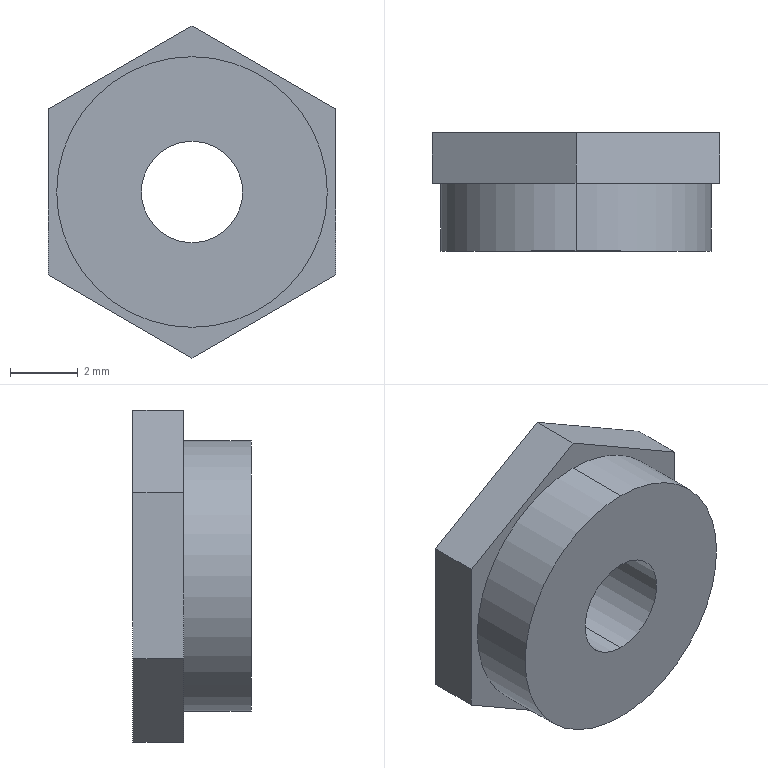Part | SolidWorks | features ICE 2, Extrusion 1 | 1 solid | 13 faces | box 8.5 x 3.5 x 9.815 mm | volume 169.646 mm3 | plane 9 | cylinder 4 | commonest cylinder face diameters 3 x2 8 x2
STEP:
#1=CARTESIAN_POINT('',(0.,0.,-1.5));
#2=VERTEX_POINT('',#1);
#3=CARTESIAN_POINT('',(0.,0.,1.5));
#4=VERTEX_POINT('',#3);
#5=CARTESIAN_POINT('',(0.,0.,0.));
#6=DIRECTION('',(0.,1.,0.));
#7=DIRECTION('',(0.,0.,1.));
#8=AXIS2_PLACEMENT_3D('',#5,#6,#7);
#9=CIRCLE('',#8,1.5);
#10=EDGE_CURVE('',#2,#4,#9,.T.);
#11=ORIENTED_EDGE('',*,*,#10,.F.);
#12=CARTESIAN_POINT('',(0.,3.5,-1.5));
#13=VERTEX_POINT('',#12);
#14=CARTESIAN_POINT('',(0.,0.,-1.5));
#15=DIRECTION('',(0.,1.,0.));
#16=VECTOR('',#15,1000.);
#17=LINE('',#14,#16);
#18=EDGE_CURVE('',#2,#13,#17,.T.);
#19=ORIENTED_EDGE('',*,*,#18,.T.);
#20=CARTESIAN_POINT('',(0.,3.5,1.5));
#21=VERTEX_POINT('',#20);
#22=CARTESIAN_POINT('',(0.,3.5,0.));
#23=DIRECTION('',(0.,1.,0.));
#24=DIRECTION('',(0.,0.,1.));
#25=AXIS2_PLACEMENT_3D('',#22,#23,#24);
#26=CIRCLE('',#25,1.5);
#27=EDGE_CURVE('',#13,#21,#26,.T.);
#28=ORIENTED_EDGE('',*,*,#27,.T.);
#29=CARTESIAN_POINT('',(0.,0.,1.5));
#30=DIRECTION('',(0.,1.,0.));
#31=VECTOR('',#30,1000.);
#32=LINE('',#29,#31);
#33=EDGE_CURVE('',#4,#21,#32,.T.);
#34=ORIENTED_EDGE('',*,*,#33,.F.);
#35=EDGE_LOOP('',(#11,#19,#28,#34));
#36=FACE_OUTER_BOUND('',#35,.T.);
#37=CARTESIAN_POINT('',(0.,0.,0.));
#38=DIRECTION('',(0.,1.,0.));
#39=DIRECTION('',(0.,0.,1.));
#40=AXIS2_PLACEMENT_3D('',#37,#38,#39);
#41=CYLINDRICAL_SURFACE('',#40,1.5);
#42=ADVANCED_FACE('',(#36),#41,.F.);
#43=CARTESIAN_POINT('',(0.,2.,4.));
#44=VERTEX_POINT('',#43);
#45=CARTESIAN_POINT('',(0.,2.,-4.));
#46=VERTEX_POINT('',#45);
#47=CARTESIAN_POINT('',(0.,2.,0.));
#48=DIRECTION('',(0.,1.,0.));
#49=DIRECTION('',(0.,0.,1.));
#50=AXIS2_PLACEMENT_3D('',#47,#48,#49);
#51=CIRCLE('',#50,4.);
#52=EDGE_CURVE('',#44,#46,#51,.T.);
#53=ORIENTED_EDGE('',*,*,#52,.F.);
#54=CARTESIAN_POINT('',(0.,0.,4.));
#55=VERTEX_POINT('',#54);
#56=CARTESIAN_POINT('',(0.,2.,4.));
#57=DIRECTION('',(0.,-1.,0.));
#58=VECTOR('',#57,1000.);
#59=LINE('',#56,#58);
#60=EDGE_CURVE('',#44,#55,#59,.T.);
#61=ORIENTED_EDGE('',*,*,#60,.T.);
#62=CARTESIAN_POINT('',(0.,0.,-4.));
#63=VERTEX_POINT('',#62);
#64=CARTESIAN_POINT('',(0.,0.,0.));
#65=DIRECTION('',(0.,1.,0.));
#66=DIRECTION('',(0.,0.,1.));
#67=AXIS2_PLACEMENT_3D('',#64,#65,#66);
#68=CIRCLE('',#67,4.);
#69=EDGE_CURVE('',#55,#63,#68,.T.);
#70=ORIENTED_EDGE('',*,*,#69,.T.);
#71=CARTESIAN_POINT('',(0.,2.,-4.));
#72=DIRECTION('',(0.,-1.,0.));
#73=VECTOR('',#72,1000.);
#74=LINE('',#71,#73);
#75=EDGE_CURVE('',#46,#63,#74,.T.);
#76=ORIENTED_EDGE('',*,*,#75,.F.);
#77=EDGE_LOOP('',(#53,#61,#70,#76));
#78=FACE_OUTER_BOUND('',#77,.T.);
#79=CARTESIAN_POINT('',(0.,2.,0.));
#80=DIRECTION('',(0.,-1.,0.));
#81=DIRECTION('',(0.,0.,-1.));
#82=AXIS2_PLACEMENT_3D('',#79,#80,#81);
#83=CYLINDRICAL_SURFACE('',#82,4.);
#84=ADVANCED_FACE('',(#78),#83,.T.);
#85=ORIENTED_EDGE('',*,*,#60,.F.);
#86=CARTESIAN_POINT('',(0.,2.,0.));
#87=DIRECTION('',(0.,1.,0.));
#88=DIRECTION('',(0.,0.,1.));
#89=AXIS2_PLACEMENT_3D('',#86,#87,#88);
#90=CIRCLE('',#89,4.);
#91=EDGE_CURVE('',#46,#44,#90,.T.);
#92=ORIENTED_EDGE('',*,*,#91,.F.);
#93=ORIENTED_EDGE('',*,*,#75,.T.);
#94=CARTESIAN_POINT('',(0.,0.,0.));
#95=DIRECTION('',(0.,1.,0.));
#96=DIRECTION('',(0.,0.,1.));
#97=AXIS2_PLACEMENT_3D('',#94,#95,#96);
#98=CIRCLE('',#97,4.);
#99=EDGE_CURVE('',#63,#55,#98,.T.);
#100=ORIENTED_EDGE('',*,*,#99,.T.);
#101=EDGE_LOOP('',(#85,#92,#93,#100));
#102=FACE_OUTER_BOUND('',#101,.T.);
#103=CARTESIAN_POINT('',(0.,2.,0.));
#104=DIRECTION('',(0.,-1.,0.));
#105=DIRECTION('',(0.,0.,-1.));
#106=AXIS2_PLACEMENT_3D('',#103,#104,#105);
#107=CYLINDRICAL_SURFACE('',#106,4.);
#108=ADVANCED_FACE('',(#102),#107,.T.);
#109=CARTESIAN_POINT('',(0.,0.,0.));
#110=DIRECTION('',(0.,1.,0.));
#111=DIRECTION('',(0.,0.,1.));
#112=AXIS2_PLACEMENT_3D('',#109,#110,#111);
#113=CIRCLE('',#112,1.5);
#114=EDGE_CURVE('',#4,#2,#113,.T.);
#115=ORIENTED_EDGE('',*,*,#114,.T.);
#116=ORIENTED_EDGE('',*,*,#10,.T.);
#117=EDGE_LOOP('',(#115,#116));
#118=FACE_BOUND('',#117,.T.);
#119=ORIENTED_EDGE('',*,*,#99,.F.);
#120=ORIENTED_EDGE('',*,*,#69,.F.);
#121=EDGE_LOOP('',(#119,#120));
#122=FACE_OUTER_BOUND('',#121,.T.);
#123=CARTESIAN_POINT('',(0.,0.,0.));
#124=DIRECTION('',(0.,1.,0.));
#125=DIRECTION('',(0.,0.,1.));
#126=AXIS2_PLACEMENT_3D('',#123,#124,#125);
#127=PLANE('',#126);
#128=ADVANCED_FACE('',(#118,#122),#127,.F.);
#129=CARTESIAN_POINT('',(4.25,2.,-2.454));
#130=VERTEX_POINT('',#129);
#131=CARTESIAN_POINT('',(0.,2.,-4.907));
#132=VERTEX_POINT('',#131);
#133=CARTESIAN_POINT('',(4.25,2.,-2.454));
#134=DIRECTION('',(-0.866,0.,-0.5));
#135=VECTOR('',#134,1000.);
#136=LINE('',#133,#135);
#137=EDGE_CURVE('',#130,#132,#136,.T.);
#138=ORIENTED_EDGE('',*,*,#137,.T.);
#139=CARTESIAN_POINT('',(0.,3.5,-4.907));
#140=VERTEX_POINT('',#139);
#141=CARTESIAN_POINT('',(0.,3.5,-4.907));
#142=DIRECTION('',(0.,-1.,0.));
#143=VECTOR('',#142,1000.);
#144=LINE('',#141,#143);
#145=EDGE_CURVE('',#140,#132,#144,.T.);
#146=ORIENTED_EDGE('',*,*,#145,.F.);
#147=CARTESIAN_POINT('',(4.25,3.5,-2.454));
#148=VERTEX_POINT('',#147);
#149=CARTESIAN_POINT('',(4.25,3.5,-2.454));
#150=DIRECTION('',(-0.866,0.,-0.5));
#151=VECTOR('',#150,1000.);
#152=LINE('',#149,#151);
#153=EDGE_CURVE('',#148,#140,#152,.T.);
#154=ORIENTED_EDGE('',*,*,#153,.F.);
#155=CARTESIAN_POINT('',(4.25,3.5,-2.454));
#156=DIRECTION('',(0.,-1.,0.));
#157=VECTOR('',#156,1000.);
#158=LINE('',#155,#157);
#159=EDGE_CURVE('',#148,#130,#158,.T.);
#160=ORIENTED_EDGE('',*,*,#159,.T.);
#161=EDGE_LOOP('',(#138,#146,#154,#160));
#162=FACE_OUTER_BOUND('',#161,.T.);
#163=CARTESIAN_POINT('',(4.25,3.5,-2.454));
#164=DIRECTION('',(-0.5,0.,0.866));
#165=DIRECTION('',(0.866,0.,0.5));
#166=AXIS2_PLACEMENT_3D('',#163,#164,#165);
#167=PLANE('',#166);
#168=ADVANCED_FACE('',(#162),#167,.F.);
#169=CARTESIAN_POINT('',(-4.25,2.,-2.454));
#170=VERTEX_POINT('',#169);
#171=CARTESIAN_POINT('',(0.,2.,-4.907));
#172=DIRECTION('',(-0.866,0.,0.5));
#173=VECTOR('',#172,1000.);
#174=LINE('',#171,#173);
#175=EDGE_CURVE('',#132,#170,#174,.T.);
#176=ORIENTED_EDGE('',*,*,#175,.T.);
#177=CARTESIAN_POINT('',(-4.25,3.5,-2.454));
#178=VERTEX_POINT('',#177);
#179=CARTESIAN_POINT('',(-4.25,3.5,-2.454));
#180=DIRECTION('',(0.,-1.,0.));
#181=VECTOR('',#180,1000.);
#182=LINE('',#179,#181);
#183=EDGE_CURVE('',#178,#170,#182,.T.);
#184=ORIENTED_EDGE('',*,*,#183,.F.);
#185=CARTESIAN_POINT('',(0.,3.5,-4.907));
#186=DIRECTION('',(-0.866,0.,0.5));
#187=VECTOR('',#186,1000.);
#188=LINE('',#185,#187);
#189=EDGE_CURVE('',#140,#178,#188,.T.);
#190=ORIENTED_EDGE('',*,*,#189,.F.);
#191=ORIENTED_EDGE('',*,*,#145,.T.);
#192=EDGE_LOOP('',(#176,#184,#190,#191));
#193=FACE_OUTER_BOUND('',#192,.T.);
#194=CARTESIAN_POINT('',(0.,3.5,-4.907));
#195=DIRECTION('',(0.5,0.,0.866));
#196=DIRECTION('',(0.866,0.,-0.5));
#197=AXIS2_PLACEMENT_3D('',#194,#195,#196);
#198=PLANE('',#197);
#199=ADVANCED_FACE('',(#193),#198,.F.);
#200=CARTESIAN_POINT('',(-4.25,2.,2.454));
#201=VERTEX_POINT('',#200);
#202=CARTESIAN_POINT('',(-4.25,2.,-2.454));
#203=DIRECTION('',(0.,0.,1.));
#204=VECTOR('',#203,1000.);
#205=LINE('',#202,#204);
#206=EDGE_CURVE('',#170,#201,#205,.T.);
#207=ORIENTED_EDGE('',*,*,#206,.T.);
#208=CARTESIAN_POINT('',(-4.25,3.5,2.454));
#209=VERTEX_POINT('',#208);
#210=CARTESIAN_POINT('',(-4.25,3.5,2.454));
#211=DIRECTION('',(0.,-1.,0.));
#212=VECTOR('',#211,1000.);
#213=LINE('',#210,#212);
#214=EDGE_CURVE('',#209,#201,#213,.T.);
#215=ORIENTED_EDGE('',*,*,#214,.F.);
#216=CARTESIAN_POINT('',(-4.25,3.5,-2.454));
#217=DIRECTION('',(0.,0.,1.));
#218=VECTOR('',#217,1000.);
#219=LINE('',#216,#218);
#220=EDGE_CURVE('',#178,#209,#219,.T.);
#221=ORIENTED_EDGE('',*,*,#220,.F.);
#222=ORIENTED_EDGE('',*,*,#183,.T.);
#223=EDGE_LOOP('',(#207,#215,#221,#222));
#224=FACE_OUTER_BOUND('',#223,.T.);
#225=CARTESIAN_POINT('',(-4.25,3.5,-2.454));
#226=DIRECTION('',(1.,0.,0.));
#227=DIRECTION('',(0.,0.,-1.));
#228=AXIS2_PLACEMENT_3D('',#225,#226,#227);
#229=PLANE('',#228);
#230=ADVANCED_FACE('',(#224),#229,.F.);
#231=CARTESIAN_POINT('',(0.,2.,4.907));
#232=VERTEX_POINT('',#231);
#233=CARTESIAN_POINT('',(-4.25,2.,2.454));
#234=DIRECTION('',(0.866,0.,0.5));
#235=VECTOR('',#234,1000.);
#236=LINE('',#233,#235);
#237=EDGE_CURVE('',#201,#232,#236,.T.);
#238=ORIENTED_EDGE('',*,*,#237,.T.);
#239=CARTESIAN_POINT('',(0.,3.5,4.907));
#240=VERTEX_POINT('',#239);
#241=CARTESIAN_POINT('',(0.,3.5,4.907));
#242=DIRECTION('',(0.,-1.,0.));
#243=VECTOR('',#242,1000.);
#244=LINE('',#241,#243);
#245=EDGE_CURVE('',#240,#232,#244,.T.);
#246=ORIENTED_EDGE('',*,*,#245,.F.);
#247=CARTESIAN_POINT('',(-4.25,3.5,2.454));
#248=DIRECTION('',(0.866,0.,0.5));
#249=VECTOR('',#248,1000.);
#250=LINE('',#247,#249);
#251=EDGE_CURVE('',#209,#240,#250,.T.);
#252=ORIENTED_EDGE('',*,*,#251,.F.);
#253=ORIENTED_EDGE('',*,*,#214,.T.);
#254=EDGE_LOOP('',(#238,#246,#252,#253));
#255=FACE_OUTER_BOUND('',#254,.T.);
#256=CARTESIAN_POINT('',(-4.25,3.5,2.454));
#257=DIRECTION('',(0.5,0.,-0.866));
#258=DIRECTION('',(-0.866,0.,-0.5));
#259=AXIS2_PLACEMENT_3D('',#256,#257,#258);
#260=PLANE('',#259);
#261=ADVANCED_FACE('',(#255),#260,.F.);
#262=CARTESIAN_POINT('',(4.25,2.,2.454));
#263=VERTEX_POINT('',#262);
#264=CARTESIAN_POINT('',(0.,2.,4.907));
#265=DIRECTION('',(0.866,0.,-0.5));
#266=VECTOR('',#265,1000.);
#267=LINE('',#264,#266);
#268=EDGE_CURVE('',#232,#263,#267,.T.);
#269=ORIENTED_EDGE('',*,*,#268,.T.);
#270=CARTESIAN_POINT('',(4.25,3.5,2.454));
#271=VERTEX_POINT('',#270);
#272=CARTESIAN_POINT('',(4.25,3.5,2.454));
#273=DIRECTION('',(0.,-1.,0.));
#274=VECTOR('',#273,1000.);
#275=LINE('',#272,#274);
#276=EDGE_CURVE('',#271,#263,#275,.T.);
#277=ORIENTED_EDGE('',*,*,#276,.F.);
#278=CARTESIAN_POINT('',(0.,3.5,4.907));
#279=DIRECTION('',(0.866,0.,-0.5));
#280=VECTOR('',#279,1000.);
#281=LINE('',#278,#280);
#282=EDGE_CURVE('',#240,#271,#281,.T.);
#283=ORIENTED_EDGE('',*,*,#282,.F.);
#284=ORIENTED_EDGE('',*,*,#245,.T.);
#285=EDGE_LOOP('',(#269,#277,#283,#284));
#286=FACE_OUTER_BOUND('',#285,.T.);
#287=CARTESIAN_POINT('',(0.,3.5,4.907));
#288=DIRECTION('',(-0.5,0.,-0.866));
#289=DIRECTION('',(-0.866,0.,0.5));
#290=AXIS2_PLACEMENT_3D('',#287,#288,#289);
#291=PLANE('',#290);
#292=ADVANCED_FACE('',(#286),#291,.F.);
#293=CARTESIAN_POINT('',(4.25,2.,2.454));
#294=DIRECTION('',(0.,0.,-1.));
#295=VECTOR('',#294,1000.);
#296=LINE('',#293,#295);
#297=EDGE_CURVE('',#263,#130,#296,.T.);
#298=ORIENTED_EDGE('',*,*,#297,.T.);
#299=ORIENTED_EDGE('',*,*,#159,.F.);
#300=CARTESIAN_POINT('',(4.25,3.5,2.454));
#301=DIRECTION('',(0.,0.,-1.));
#302=VECTOR('',#301,1000.);
#303=LINE('',#300,#302);
#304=EDGE_CURVE('',#271,#148,#303,.T.);
#305=ORIENTED_EDGE('',*,*,#304,.F.);
#306=ORIENTED_EDGE('',*,*,#276,.T.);
#307=EDGE_LOOP('',(#298,#299,#305,#306));
#308=FACE_OUTER_BOUND('',#307,.T.);
#309=CARTESIAN_POINT('',(4.25,3.5,2.454));
#310=DIRECTION('',(-1.,0.,0.));
#311=DIRECTION('',(0.,0.,1.));
#312=AXIS2_PLACEMENT_3D('',#309,#310,#311);
#313=PLANE('',#312);
#314=ADVANCED_FACE('',(#308),#313,.F.);
#315=CARTESIAN_POINT('',(0.,3.5,0.));
#316=DIRECTION('',(0.,1.,0.));
#317=DIRECTION('',(0.,0.,1.));
#318=AXIS2_PLACEMENT_3D('',#315,#316,#317);
#319=CIRCLE('',#318,1.5);
#320=EDGE_CURVE('',#21,#13,#319,.T.);
#321=ORIENTED_EDGE('',*,*,#320,.F.);
#322=ORIENTED_EDGE('',*,*,#27,.F.);
#323=EDGE_LOOP('',(#321,#322));
#324=FACE_BOUND('',#323,.T.);
#325=ORIENTED_EDGE('',*,*,#153,.T.);
#326=ORIENTED_EDGE('',*,*,#189,.T.);
#327=ORIENTED_EDGE('',*,*,#220,.T.);
#328=ORIENTED_EDGE('',*,*,#251,.T.);
#329=ORIENTED_EDGE('',*,*,#282,.T.);
#330=ORIENTED_EDGE('',*,*,#304,.T.);
#331=EDGE_LOOP('',(#325,#326,#327,#328,#329,#330));
#332=FACE_OUTER_BOUND('',#331,.T.);
#333=CARTESIAN_POINT('',(0.,3.5,0.));
#334=DIRECTION('',(0.,1.,0.));
#335=DIRECTION('',(0.,0.,1.));
#336=AXIS2_PLACEMENT_3D('',#333,#334,#335);
#337=PLANE('',#336);
#338=ADVANCED_FACE('',(#324,#332),#337,.T.);
#339=ORIENTED_EDGE('',*,*,#91,.T.);
#340=ORIENTED_EDGE('',*,*,#52,.T.);
#341=EDGE_LOOP('',(#339,#340));
#342=FACE_BOUND('',#341,.T.);
#343=ORIENTED_EDGE('',*,*,#137,.F.);
#344=ORIENTED_EDGE('',*,*,#297,.F.);
#345=ORIENTED_EDGE('',*,*,#268,.F.);
#346=ORIENTED_EDGE('',*,*,#237,.F.);
#347=ORIENTED_EDGE('',*,*,#206,.F.);
#348=ORIENTED_EDGE('',*,*,#175,.F.);
#349=EDGE_LOOP('',(#343,#344,#345,#346,#347,#348));
#350=FACE_OUTER_BOUND('',#349,.T.);
#351=CARTESIAN_POINT('',(0.,2.,0.));
#352=DIRECTION('',(0.,1.,0.));
#353=DIRECTION('',(0.,0.,1.));
#354=AXIS2_PLACEMENT_3D('',#351,#352,#353);
#355=PLANE('',#354);
#356=ADVANCED_FACE('',(#342,#350),#355,.F.);
#357=ORIENTED_EDGE('',*,*,#18,.F.);
#358=ORIENTED_EDGE('',*,*,#114,.F.);
#359=ORIENTED_EDGE('',*,*,#33,.T.);
#360=ORIENTED_EDGE('',*,*,#320,.T.);
#361=EDGE_LOOP('',(#357,#358,#359,#360));
#362=FACE_OUTER_BOUND('',#361,.T.);
#363=CARTESIAN_POINT('',(0.,0.,0.));
#364=DIRECTION('',(0.,1.,0.));
#365=DIRECTION('',(0.,0.,1.));
#366=AXIS2_PLACEMENT_3D('',#363,#364,#365);
#367=CYLINDRICAL_SURFACE('',#366,1.5);
#368=ADVANCED_FACE('',(#362),#367,.F.);
#369=CLOSED_SHELL('',(#42,#84,#108,#128,#168,#199,#230,#261,#292,#314,#338,#356,#368));
#370=MANIFOLD_SOLID_BREP('',#369);
#371=CARTESIAN_POINT('',(0.,0.,0.));
#372=DIRECTION('',(0.,0.,1.));
#373=DIRECTION('',(1.,0.,0.));
#374=AXIS2_PLACEMENT_3D('',#371,#372,#373);
#375=(LENGTH_UNIT()NAMED_UNIT(*)SI_UNIT(.MILLI.,.METRE.));
#376=UNCERTAINTY_MEASURE_WITH_UNIT(LENGTH_MEASURE(0.00001),#375,'','');
#377=(NAMED_UNIT(*)PLANE_ANGLE_UNIT()SI_UNIT($,.RADIAN.));
#378=(NAMED_UNIT(*)SI_UNIT($,.STERADIAN.)SOLID_ANGLE_UNIT());
#379=(GEOMETRIC_REPRESENTATION_CONTEXT(3)GLOBAL_UNCERTAINTY_ASSIGNED_CONTEXT((#376))GLOBAL_UNIT_ASSIGNED_CONTEXT((#375,#377,#378))REPRESENTATION_CONTEXT('',''));
#380=ADVANCED_BREP_SHAPE_REPRESENTATION('',(#370,#374),#379);